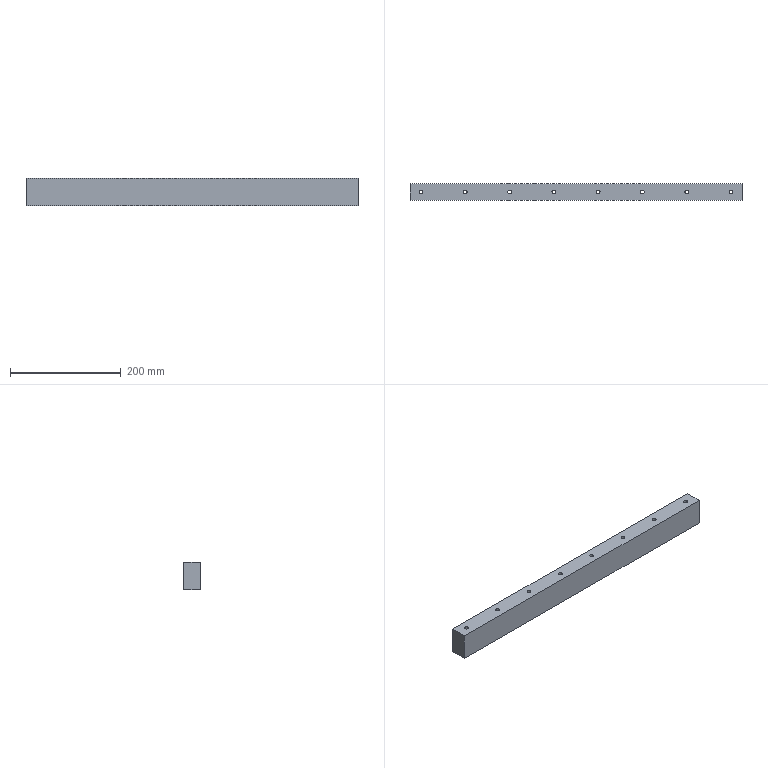Part | SolidWorks | features 3DProfileFeature 1, BaseBody 1, HoleWzd 1, LPattern 1 | 1 solid | 22 faces | box 600 x 30 x 50 mm | volume 885473 mm3 | cylinder 16 | plane 6 | commonest cylinder face diameters 6.8 x16
STEP:
#1=CARTESIAN_POINT('',(-276.6,0.,-25.));
#2=VERTEX_POINT('',#1);
#3=CARTESIAN_POINT('',(-283.4,0.,-25.));
#4=VERTEX_POINT('',#3);
#5=CARTESIAN_POINT('',(-280.,0.,-25.));
#6=DIRECTION('',(0.,0.,-1.));
#7=DIRECTION('',(1.,0.,0.));
#8=AXIS2_PLACEMENT_3D('',#5,#6,#7);
#9=CIRCLE('',#8,3.4);
#10=EDGE_CURVE('',#2,#4,#9,.T.);
#11=ORIENTED_EDGE('',*,*,#10,.T.);
#12=CARTESIAN_POINT('',(-283.4,0.,25.));
#13=VERTEX_POINT('',#12);
#14=CARTESIAN_POINT('',(-283.4,0.,-25.));
#15=DIRECTION('',(0.,0.,1.));
#16=VECTOR('',#15,1000.);
#17=LINE('',#14,#16);
#18=EDGE_CURVE('',#4,#13,#17,.T.);
#19=ORIENTED_EDGE('',*,*,#18,.T.);
#20=CARTESIAN_POINT('',(-276.6,0.,25.));
#21=VERTEX_POINT('',#20);
#22=CARTESIAN_POINT('',(-280.,0.,25.));
#23=DIRECTION('',(0.,0.,1.));
#24=DIRECTION('',(1.,0.,0.));
#25=AXIS2_PLACEMENT_3D('',#22,#23,#24);
#26=CIRCLE('',#25,3.4);
#27=EDGE_CURVE('',#13,#21,#26,.T.);
#28=ORIENTED_EDGE('',*,*,#27,.T.);
#29=CARTESIAN_POINT('',(-276.6,0.,-25.));
#30=DIRECTION('',(0.,0.,1.));
#31=VECTOR('',#30,1000.);
#32=LINE('',#29,#31);
#33=EDGE_CURVE('',#2,#21,#32,.T.);
#34=ORIENTED_EDGE('',*,*,#33,.F.);
#35=EDGE_LOOP('',(#11,#19,#28,#34));
#36=FACE_OUTER_BOUND('',#35,.T.);
#37=CARTESIAN_POINT('',(-280.,0.,-25.));
#38=DIRECTION('',(0.,0.,1.));
#39=DIRECTION('',(1.,0.,0.));
#40=AXIS2_PLACEMENT_3D('',#37,#38,#39);
#41=CYLINDRICAL_SURFACE('',#40,3.4);
#42=ADVANCED_FACE('',(#36),#41,.F.);
#43=CARTESIAN_POINT('',(276.6,0.,-25.));
#44=VERTEX_POINT('',#43);
#45=CARTESIAN_POINT('',(283.4,0.,-25.));
#46=VERTEX_POINT('',#45);
#47=CARTESIAN_POINT('',(280.,0.,-25.));
#48=DIRECTION('',(0.,0.,1.));
#49=DIRECTION('',(1.,0.,0.));
#50=AXIS2_PLACEMENT_3D('',#47,#48,#49);
#51=CIRCLE('',#50,3.4);
#52=EDGE_CURVE('',#44,#46,#51,.T.);
#53=ORIENTED_EDGE('',*,*,#52,.F.);
#54=CARTESIAN_POINT('',(276.6,0.,25.));
#55=VERTEX_POINT('',#54);
#56=CARTESIAN_POINT('',(276.6,0.,-25.));
#57=DIRECTION('',(0.,0.,1.));
#58=VECTOR('',#57,1000.);
#59=LINE('',#56,#58);
#60=EDGE_CURVE('',#44,#55,#59,.T.);
#61=ORIENTED_EDGE('',*,*,#60,.T.);
#62=CARTESIAN_POINT('',(283.4,0.,25.));
#63=VERTEX_POINT('',#62);
#64=CARTESIAN_POINT('',(280.,0.,25.));
#65=DIRECTION('',(0.,0.,1.));
#66=DIRECTION('',(1.,0.,0.));
#67=AXIS2_PLACEMENT_3D('',#64,#65,#66);
#68=CIRCLE('',#67,3.4);
#69=EDGE_CURVE('',#55,#63,#68,.T.);
#70=ORIENTED_EDGE('',*,*,#69,.T.);
#71=CARTESIAN_POINT('',(283.4,0.,-25.));
#72=DIRECTION('',(0.,0.,1.));
#73=VECTOR('',#72,1000.);
#74=LINE('',#71,#73);
#75=EDGE_CURVE('',#46,#63,#74,.T.);
#76=ORIENTED_EDGE('',*,*,#75,.F.);
#77=EDGE_LOOP('',(#53,#61,#70,#76));
#78=FACE_OUTER_BOUND('',#77,.T.);
#79=CARTESIAN_POINT('',(280.,0.,-25.));
#80=DIRECTION('',(0.,0.,1.));
#81=DIRECTION('',(1.,0.,0.));
#82=AXIS2_PLACEMENT_3D('',#79,#80,#81);
#83=CYLINDRICAL_SURFACE('',#82,3.4);
#84=ADVANCED_FACE('',(#78),#83,.F.);
#85=CARTESIAN_POINT('',(196.6,0.,-25.));
#86=VERTEX_POINT('',#85);
#87=CARTESIAN_POINT('',(203.4,0.,-25.));
#88=VERTEX_POINT('',#87);
#89=CARTESIAN_POINT('',(200.,0.,-25.));
#90=DIRECTION('',(0.,0.,1.));
#91=DIRECTION('',(1.,0.,0.));
#92=AXIS2_PLACEMENT_3D('',#89,#90,#91);
#93=CIRCLE('',#92,3.4);
#94=EDGE_CURVE('',#86,#88,#93,.T.);
#95=ORIENTED_EDGE('',*,*,#94,.F.);
#96=CARTESIAN_POINT('',(196.6,0.,25.));
#97=VERTEX_POINT('',#96);
#98=CARTESIAN_POINT('',(196.6,0.,-25.));
#99=DIRECTION('',(0.,0.,1.));
#100=VECTOR('',#99,1000.);
#101=LINE('',#98,#100);
#102=EDGE_CURVE('',#86,#97,#101,.T.);
#103=ORIENTED_EDGE('',*,*,#102,.T.);
#104=CARTESIAN_POINT('',(203.4,0.,25.));
#105=VERTEX_POINT('',#104);
#106=CARTESIAN_POINT('',(200.,0.,25.));
#107=DIRECTION('',(0.,0.,1.));
#108=DIRECTION('',(1.,0.,0.));
#109=AXIS2_PLACEMENT_3D('',#106,#107,#108);
#110=CIRCLE('',#109,3.4);
#111=EDGE_CURVE('',#97,#105,#110,.T.);
#112=ORIENTED_EDGE('',*,*,#111,.T.);
#113=CARTESIAN_POINT('',(203.4,0.,-25.));
#114=DIRECTION('',(0.,0.,1.));
#115=VECTOR('',#114,1000.);
#116=LINE('',#113,#115);
#117=EDGE_CURVE('',#88,#105,#116,.T.);
#118=ORIENTED_EDGE('',*,*,#117,.F.);
#119=EDGE_LOOP('',(#95,#103,#112,#118));
#120=FACE_OUTER_BOUND('',#119,.T.);
#121=CARTESIAN_POINT('',(200.,0.,-25.));
#122=DIRECTION('',(0.,0.,1.));
#123=DIRECTION('',(1.,0.,0.));
#124=AXIS2_PLACEMENT_3D('',#121,#122,#123);
#125=CYLINDRICAL_SURFACE('',#124,3.4);
#126=ADVANCED_FACE('',(#120),#125,.F.);
#127=CARTESIAN_POINT('',(116.6,0.,-25.));
#128=VERTEX_POINT('',#127);
#129=CARTESIAN_POINT('',(123.4,0.,-25.));
#130=VERTEX_POINT('',#129);
#131=CARTESIAN_POINT('',(120.,0.,-25.));
#132=DIRECTION('',(0.,0.,1.));
#133=DIRECTION('',(1.,0.,0.));
#134=AXIS2_PLACEMENT_3D('',#131,#132,#133);
#135=CIRCLE('',#134,3.4);
#136=EDGE_CURVE('',#128,#130,#135,.T.);
#137=ORIENTED_EDGE('',*,*,#136,.F.);
#138=CARTESIAN_POINT('',(116.6,0.,25.));
#139=VERTEX_POINT('',#138);
#140=CARTESIAN_POINT('',(116.6,0.,-25.));
#141=DIRECTION('',(0.,0.,1.));
#142=VECTOR('',#141,1000.);
#143=LINE('',#140,#142);
#144=EDGE_CURVE('',#128,#139,#143,.T.);
#145=ORIENTED_EDGE('',*,*,#144,.T.);
#146=CARTESIAN_POINT('',(123.4,0.,25.));
#147=VERTEX_POINT('',#146);
#148=CARTESIAN_POINT('',(120.,0.,25.));
#149=DIRECTION('',(0.,0.,1.));
#150=DIRECTION('',(1.,0.,0.));
#151=AXIS2_PLACEMENT_3D('',#148,#149,#150);
#152=CIRCLE('',#151,3.4);
#153=EDGE_CURVE('',#139,#147,#152,.T.);
#154=ORIENTED_EDGE('',*,*,#153,.T.);
#155=CARTESIAN_POINT('',(123.4,0.,-25.));
#156=DIRECTION('',(0.,0.,1.));
#157=VECTOR('',#156,1000.);
#158=LINE('',#155,#157);
#159=EDGE_CURVE('',#130,#147,#158,.T.);
#160=ORIENTED_EDGE('',*,*,#159,.F.);
#161=EDGE_LOOP('',(#137,#145,#154,#160));
#162=FACE_OUTER_BOUND('',#161,.T.);
#163=CARTESIAN_POINT('',(120.,0.,-25.));
#164=DIRECTION('',(0.,0.,1.));
#165=DIRECTION('',(1.,0.,0.));
#166=AXIS2_PLACEMENT_3D('',#163,#164,#165);
#167=CYLINDRICAL_SURFACE('',#166,3.4);
#168=ADVANCED_FACE('',(#162),#167,.F.);
#169=CARTESIAN_POINT('',(36.6,0.,-25.));
#170=VERTEX_POINT('',#169);
#171=CARTESIAN_POINT('',(43.4,0.,-25.));
#172=VERTEX_POINT('',#171);
#173=CARTESIAN_POINT('',(40.,0.,-25.));
#174=DIRECTION('',(0.,0.,1.));
#175=DIRECTION('',(1.,0.,0.));
#176=AXIS2_PLACEMENT_3D('',#173,#174,#175);
#177=CIRCLE('',#176,3.4);
#178=EDGE_CURVE('',#170,#172,#177,.T.);
#179=ORIENTED_EDGE('',*,*,#178,.F.);
#180=CARTESIAN_POINT('',(36.6,0.,25.));
#181=VERTEX_POINT('',#180);
#182=CARTESIAN_POINT('',(36.6,0.,-25.));
#183=DIRECTION('',(0.,0.,1.));
#184=VECTOR('',#183,1000.);
#185=LINE('',#182,#184);
#186=EDGE_CURVE('',#170,#181,#185,.T.);
#187=ORIENTED_EDGE('',*,*,#186,.T.);
#188=CARTESIAN_POINT('',(43.4,0.,25.));
#189=VERTEX_POINT('',#188);
#190=CARTESIAN_POINT('',(40.,0.,25.));
#191=DIRECTION('',(0.,0.,1.));
#192=DIRECTION('',(1.,0.,0.));
#193=AXIS2_PLACEMENT_3D('',#190,#191,#192);
#194=CIRCLE('',#193,3.4);
#195=EDGE_CURVE('',#181,#189,#194,.T.);
#196=ORIENTED_EDGE('',*,*,#195,.T.);
#197=CARTESIAN_POINT('',(43.4,0.,-25.));
#198=DIRECTION('',(0.,0.,1.));
#199=VECTOR('',#198,1000.);
#200=LINE('',#197,#199);
#201=EDGE_CURVE('',#172,#189,#200,.T.);
#202=ORIENTED_EDGE('',*,*,#201,.F.);
#203=EDGE_LOOP('',(#179,#187,#196,#202));
#204=FACE_OUTER_BOUND('',#203,.T.);
#205=CARTESIAN_POINT('',(40.,0.,-25.));
#206=DIRECTION('',(0.,0.,1.));
#207=DIRECTION('',(1.,0.,0.));
#208=AXIS2_PLACEMENT_3D('',#205,#206,#207);
#209=CYLINDRICAL_SURFACE('',#208,3.4);
#210=ADVANCED_FACE('',(#204),#209,.F.);
#211=CARTESIAN_POINT('',(-43.4,0.,-25.));
#212=VERTEX_POINT('',#211);
#213=CARTESIAN_POINT('',(-36.6,0.,-25.));
#214=VERTEX_POINT('',#213);
#215=CARTESIAN_POINT('',(-40.,0.,-25.));
#216=DIRECTION('',(0.,0.,1.));
#217=DIRECTION('',(1.,0.,0.));
#218=AXIS2_PLACEMENT_3D('',#215,#216,#217);
#219=CIRCLE('',#218,3.4);
#220=EDGE_CURVE('',#212,#214,#219,.T.);
#221=ORIENTED_EDGE('',*,*,#220,.F.);
#222=CARTESIAN_POINT('',(-43.4,0.,25.));
#223=VERTEX_POINT('',#222);
#224=CARTESIAN_POINT('',(-43.4,0.,-25.));
#225=DIRECTION('',(0.,0.,1.));
#226=VECTOR('',#225,1000.);
#227=LINE('',#224,#226);
#228=EDGE_CURVE('',#212,#223,#227,.T.);
#229=ORIENTED_EDGE('',*,*,#228,.T.);
#230=CARTESIAN_POINT('',(-36.6,0.,25.));
#231=VERTEX_POINT('',#230);
#232=CARTESIAN_POINT('',(-40.,0.,25.));
#233=DIRECTION('',(0.,0.,1.));
#234=DIRECTION('',(1.,0.,0.));
#235=AXIS2_PLACEMENT_3D('',#232,#233,#234);
#236=CIRCLE('',#235,3.4);
#237=EDGE_CURVE('',#223,#231,#236,.T.);
#238=ORIENTED_EDGE('',*,*,#237,.T.);
#239=CARTESIAN_POINT('',(-36.6,0.,-25.));
#240=DIRECTION('',(0.,0.,1.));
#241=VECTOR('',#240,1000.);
#242=LINE('',#239,#241);
#243=EDGE_CURVE('',#214,#231,#242,.T.);
#244=ORIENTED_EDGE('',*,*,#243,.F.);
#245=EDGE_LOOP('',(#221,#229,#238,#244));
#246=FACE_OUTER_BOUND('',#245,.T.);
#247=CARTESIAN_POINT('',(-40.,0.,-25.));
#248=DIRECTION('',(0.,0.,1.));
#249=DIRECTION('',(1.,0.,0.));
#250=AXIS2_PLACEMENT_3D('',#247,#248,#249);
#251=CYLINDRICAL_SURFACE('',#250,3.4);
#252=ADVANCED_FACE('',(#246),#251,.F.);
#253=CARTESIAN_POINT('',(-123.4,0.,-25.));
#254=VERTEX_POINT('',#253);
#255=CARTESIAN_POINT('',(-116.6,0.,-25.));
#256=VERTEX_POINT('',#255);
#257=CARTESIAN_POINT('',(-120.,0.,-25.));
#258=DIRECTION('',(0.,0.,1.));
#259=DIRECTION('',(1.,0.,0.));
#260=AXIS2_PLACEMENT_3D('',#257,#258,#259);
#261=CIRCLE('',#260,3.4);
#262=EDGE_CURVE('',#254,#256,#261,.T.);
#263=ORIENTED_EDGE('',*,*,#262,.F.);
#264=CARTESIAN_POINT('',(-123.4,0.,25.));
#265=VERTEX_POINT('',#264);
#266=CARTESIAN_POINT('',(-123.4,0.,-25.));
#267=DIRECTION('',(0.,0.,1.));
#268=VECTOR('',#267,1000.);
#269=LINE('',#266,#268);
#270=EDGE_CURVE('',#254,#265,#269,.T.);
#271=ORIENTED_EDGE('',*,*,#270,.T.);
#272=CARTESIAN_POINT('',(-116.6,0.,25.));
#273=VERTEX_POINT('',#272);
#274=CARTESIAN_POINT('',(-120.,0.,25.));
#275=DIRECTION('',(0.,0.,1.));
#276=DIRECTION('',(1.,0.,0.));
#277=AXIS2_PLACEMENT_3D('',#274,#275,#276);
#278=CIRCLE('',#277,3.4);
#279=EDGE_CURVE('',#265,#273,#278,.T.);
#280=ORIENTED_EDGE('',*,*,#279,.T.);
#281=CARTESIAN_POINT('',(-116.6,0.,-25.));
#282=DIRECTION('',(0.,0.,1.));
#283=VECTOR('',#282,1000.);
#284=LINE('',#281,#283);
#285=EDGE_CURVE('',#256,#273,#284,.T.);
#286=ORIENTED_EDGE('',*,*,#285,.F.);
#287=EDGE_LOOP('',(#263,#271,#280,#286));
#288=FACE_OUTER_BOUND('',#287,.T.);
#289=CARTESIAN_POINT('',(-120.,0.,-25.));
#290=DIRECTION('',(0.,0.,1.));
#291=DIRECTION('',(1.,0.,0.));
#292=AXIS2_PLACEMENT_3D('',#289,#290,#291);
#293=CYLINDRICAL_SURFACE('',#292,3.4);
#294=ADVANCED_FACE('',(#288),#293,.F.);
#295=CARTESIAN_POINT('',(-203.4,0.,-25.));
#296=VERTEX_POINT('',#295);
#297=CARTESIAN_POINT('',(-196.6,0.,-25.));
#298=VERTEX_POINT('',#297);
#299=CARTESIAN_POINT('',(-200.,0.,-25.));
#300=DIRECTION('',(0.,0.,1.));
#301=DIRECTION('',(1.,0.,0.));
#302=AXIS2_PLACEMENT_3D('',#299,#300,#301);
#303=CIRCLE('',#302,3.4);
#304=EDGE_CURVE('',#296,#298,#303,.T.);
#305=ORIENTED_EDGE('',*,*,#304,.F.);
#306=CARTESIAN_POINT('',(-203.4,0.,25.));
#307=VERTEX_POINT('',#306);
#308=CARTESIAN_POINT('',(-203.4,0.,-25.));
#309=DIRECTION('',(0.,0.,1.));
#310=VECTOR('',#309,1000.);
#311=LINE('',#308,#310);
#312=EDGE_CURVE('',#296,#307,#311,.T.);
#313=ORIENTED_EDGE('',*,*,#312,.T.);
#314=CARTESIAN_POINT('',(-196.6,0.,25.));
#315=VERTEX_POINT('',#314);
#316=CARTESIAN_POINT('',(-200.,0.,25.));
#317=DIRECTION('',(0.,0.,1.));
#318=DIRECTION('',(1.,0.,0.));
#319=AXIS2_PLACEMENT_3D('',#316,#317,#318);
#320=CIRCLE('',#319,3.4);
#321=EDGE_CURVE('',#307,#315,#320,.T.);
#322=ORIENTED_EDGE('',*,*,#321,.T.);
#323=CARTESIAN_POINT('',(-196.6,0.,-25.));
#324=DIRECTION('',(0.,0.,1.));
#325=VECTOR('',#324,1000.);
#326=LINE('',#323,#325);
#327=EDGE_CURVE('',#298,#315,#326,.T.);
#328=ORIENTED_EDGE('',*,*,#327,.F.);
#329=EDGE_LOOP('',(#305,#313,#322,#328));
#330=FACE_OUTER_BOUND('',#329,.T.);
#331=CARTESIAN_POINT('',(-200.,0.,-25.));
#332=DIRECTION('',(0.,0.,1.));
#333=DIRECTION('',(1.,0.,0.));
#334=AXIS2_PLACEMENT_3D('',#331,#332,#333);
#335=CYLINDRICAL_SURFACE('',#334,3.4);
#336=ADVANCED_FACE('',(#330),#335,.F.);
#337=ORIENTED_EDGE('',*,*,#18,.F.);
#338=CARTESIAN_POINT('',(-280.,0.,-25.));
#339=DIRECTION('',(0.,0.,-1.));
#340=DIRECTION('',(1.,0.,0.));
#341=AXIS2_PLACEMENT_3D('',#338,#339,#340);
#342=CIRCLE('',#341,3.4);
#343=EDGE_CURVE('',#4,#2,#342,.T.);
#344=ORIENTED_EDGE('',*,*,#343,.T.);
#345=ORIENTED_EDGE('',*,*,#33,.T.);
#346=CARTESIAN_POINT('',(-280.,0.,25.));
#347=DIRECTION('',(0.,0.,1.));
#348=DIRECTION('',(1.,0.,0.));
#349=AXIS2_PLACEMENT_3D('',#346,#347,#348);
#350=CIRCLE('',#349,3.4);
#351=EDGE_CURVE('',#21,#13,#350,.T.);
#352=ORIENTED_EDGE('',*,*,#351,.T.);
#353=EDGE_LOOP('',(#337,#344,#345,#352));
#354=FACE_OUTER_BOUND('',#353,.T.);
#355=CARTESIAN_POINT('',(-280.,0.,-25.));
#356=DIRECTION('',(0.,0.,1.));
#357=DIRECTION('',(1.,0.,0.));
#358=AXIS2_PLACEMENT_3D('',#355,#356,#357);
#359=CYLINDRICAL_SURFACE('',#358,3.4);
#360=ADVANCED_FACE('',(#354),#359,.F.);
#361=CARTESIAN_POINT('',(280.,0.,25.));
#362=DIRECTION('',(0.,0.,1.));
#363=DIRECTION('',(1.,0.,0.));
#364=AXIS2_PLACEMENT_3D('',#361,#362,#363);
#365=CIRCLE('',#364,3.4);
#366=EDGE_CURVE('',#63,#55,#365,.T.);
#367=ORIENTED_EDGE('',*,*,#366,.F.);
#368=ORIENTED_EDGE('',*,*,#69,.F.);
#369=EDGE_LOOP('',(#367,#368));
#370=FACE_BOUND('',#369,.T.);
#371=CARTESIAN_POINT('',(200.,0.,25.));
#372=DIRECTION('',(0.,0.,1.));
#373=DIRECTION('',(1.,0.,0.));
#374=AXIS2_PLACEMENT_3D('',#371,#372,#373);
#375=CIRCLE('',#374,3.4);
#376=EDGE_CURVE('',#105,#97,#375,.T.);
#377=ORIENTED_EDGE('',*,*,#376,.F.);
#378=ORIENTED_EDGE('',*,*,#111,.F.);
#379=EDGE_LOOP('',(#377,#378));
#380=FACE_BOUND('',#379,.T.);
#381=CARTESIAN_POINT('',(120.,0.,25.));
#382=DIRECTION('',(0.,0.,1.));
#383=DIRECTION('',(1.,0.,0.));
#384=AXIS2_PLACEMENT_3D('',#381,#382,#383);
#385=CIRCLE('',#384,3.4);
#386=EDGE_CURVE('',#147,#139,#385,.T.);
#387=ORIENTED_EDGE('',*,*,#386,.F.);
#388=ORIENTED_EDGE('',*,*,#153,.F.);
#389=EDGE_LOOP('',(#387,#388));
#390=FACE_BOUND('',#389,.T.);
#391=CARTESIAN_POINT('',(40.,0.,25.));
#392=DIRECTION('',(0.,0.,1.));
#393=DIRECTION('',(1.,0.,0.));
#394=AXIS2_PLACEMENT_3D('',#391,#392,#393);
#395=CIRCLE('',#394,3.4);
#396=EDGE_CURVE('',#189,#181,#395,.T.);
#397=ORIENTED_EDGE('',*,*,#396,.F.);
#398=ORIENTED_EDGE('',*,*,#195,.F.);
#399=EDGE_LOOP('',(#397,#398));
#400=FACE_BOUND('',#399,.T.);
#401=CARTESIAN_POINT('',(-40.,0.,25.));
#402=DIRECTION('',(0.,0.,1.));
#403=DIRECTION('',(1.,0.,0.));
#404=AXIS2_PLACEMENT_3D('',#401,#402,#403);
#405=CIRCLE('',#404,3.4);
#406=EDGE_CURVE('',#231,#223,#405,.T.);
#407=ORIENTED_EDGE('',*,*,#406,.F.);
#408=ORIENTED_EDGE('',*,*,#237,.F.);
#409=EDGE_LOOP('',(#407,#408));
#410=FACE_BOUND('',#409,.T.);
#411=CARTESIAN_POINT('',(-120.,0.,25.));
#412=DIRECTION('',(0.,0.,1.));
#413=DIRECTION('',(1.,0.,0.));
#414=AXIS2_PLACEMENT_3D('',#411,#412,#413);
#415=CIRCLE('',#414,3.4);
#416=EDGE_CURVE('',#273,#265,#415,.T.);
#417=ORIENTED_EDGE('',*,*,#416,.F.);
#418=ORIENTED_EDGE('',*,*,#279,.F.);
#419=EDGE_LOOP('',(#417,#418));
#420=FACE_BOUND('',#419,.T.);
#421=CARTESIAN_POINT('',(-200.,0.,25.));
#422=DIRECTION('',(0.,0.,1.));
#423=DIRECTION('',(1.,0.,0.));
#424=AXIS2_PLACEMENT_3D('',#421,#422,#423);
#425=CIRCLE('',#424,3.4);
#426=EDGE_CURVE('',#315,#307,#425,.T.);
#427=ORIENTED_EDGE('',*,*,#426,.F.);
#428=ORIENTED_EDGE('',*,*,#321,.F.);
#429=EDGE_LOOP('',(#427,#428));
#430=FACE_BOUND('',#429,.T.);
#431=ORIENTED_EDGE('',*,*,#351,.F.);
#432=ORIENTED_EDGE('',*,*,#27,.F.);
#433=EDGE_LOOP('',(#431,#432));
#434=FACE_BOUND('',#433,.T.);
#435=CARTESIAN_POINT('',(-300.,15.,25.));
#436=VERTEX_POINT('',#435);
#437=CARTESIAN_POINT('',(300.,15.,25.));
#438=VERTEX_POINT('',#437);
#439=CARTESIAN_POINT('',(0.,15.,25.));
#440=DIRECTION('',(1.,0.,0.));
#441=VECTOR('',#440,1000.);
#442=LINE('',#439,#441);
#443=EDGE_CURVE('',#436,#438,#442,.T.);
#444=ORIENTED_EDGE('',*,*,#443,.F.);
#445=CARTESIAN_POINT('',(-300.,-15.,25.));
#446=VERTEX_POINT('',#445);
#447=CARTESIAN_POINT('',(-300.,0.,25.));
#448=DIRECTION('',(0.,1.,0.));
#449=VECTOR('',#448,1000.);
#450=LINE('',#447,#449);
#451=EDGE_CURVE('',#446,#436,#450,.T.);
#452=ORIENTED_EDGE('',*,*,#451,.F.);
#453=CARTESIAN_POINT('',(300.,-15.,25.));
#454=VERTEX_POINT('',#453);
#455=CARTESIAN_POINT('',(0.,-15.,25.));
#456=DIRECTION('',(-1.,0.,0.));
#457=VECTOR('',#456,1000.);
#458=LINE('',#455,#457);
#459=EDGE_CURVE('',#454,#446,#458,.T.);
#460=ORIENTED_EDGE('',*,*,#459,.F.);
#461=CARTESIAN_POINT('',(300.,0.,25.));
#462=DIRECTION('',(0.,-1.,0.));
#463=VECTOR('',#462,1000.);
#464=LINE('',#461,#463);
#465=EDGE_CURVE('',#438,#454,#464,.T.);
#466=ORIENTED_EDGE('',*,*,#465,.F.);
#467=EDGE_LOOP('',(#444,#452,#460,#466));
#468=FACE_OUTER_BOUND('',#467,.T.);
#469=CARTESIAN_POINT('',(300.,-15.,25.));
#470=DIRECTION('',(0.,0.,-1.));
#471=DIRECTION('',(-1.,0.,0.));
#472=AXIS2_PLACEMENT_3D('',#469,#470,#471);
#473=PLANE('',#472);
#474=ADVANCED_FACE('',(#370,#380,#390,#400,#410,#420,#430,#434,#468),#473,.F.);
#475=CARTESIAN_POINT('',(280.,0.,-25.));
#476=DIRECTION('',(0.,0.,1.));
#477=DIRECTION('',(1.,0.,0.));
#478=AXIS2_PLACEMENT_3D('',#475,#476,#477);
#479=CIRCLE('',#478,3.4);
#480=EDGE_CURVE('',#46,#44,#479,.T.);
#481=ORIENTED_EDGE('',*,*,#480,.T.);
#482=ORIENTED_EDGE('',*,*,#52,.T.);
#483=EDGE_LOOP('',(#481,#482));
#484=FACE_BOUND('',#483,.T.);
#485=CARTESIAN_POINT('',(200.,0.,-25.));
#486=DIRECTION('',(0.,0.,1.));
#487=DIRECTION('',(1.,0.,0.));
#488=AXIS2_PLACEMENT_3D('',#485,#486,#487);
#489=CIRCLE('',#488,3.4);
#490=EDGE_CURVE('',#88,#86,#489,.T.);
#491=ORIENTED_EDGE('',*,*,#490,.T.);
#492=ORIENTED_EDGE('',*,*,#94,.T.);
#493=EDGE_LOOP('',(#491,#492));
#494=FACE_BOUND('',#493,.T.);
#495=CARTESIAN_POINT('',(120.,0.,-25.));
#496=DIRECTION('',(0.,0.,1.));
#497=DIRECTION('',(1.,0.,0.));
#498=AXIS2_PLACEMENT_3D('',#495,#496,#497);
#499=CIRCLE('',#498,3.4);
#500=EDGE_CURVE('',#130,#128,#499,.T.);
#501=ORIENTED_EDGE('',*,*,#500,.T.);
#502=ORIENTED_EDGE('',*,*,#136,.T.);
#503=EDGE_LOOP('',(#501,#502));
#504=FACE_BOUND('',#503,.T.);
#505=CARTESIAN_POINT('',(40.,0.,-25.));
#506=DIRECTION('',(0.,0.,1.));
#507=DIRECTION('',(1.,0.,0.));
#508=AXIS2_PLACEMENT_3D('',#505,#506,#507);
#509=CIRCLE('',#508,3.4);
#510=EDGE_CURVE('',#172,#170,#509,.T.);
#511=ORIENTED_EDGE('',*,*,#510,.T.);
#512=ORIENTED_EDGE('',*,*,#178,.T.);
#513=EDGE_LOOP('',(#511,#512));
#514=FACE_BOUND('',#513,.T.);
#515=CARTESIAN_POINT('',(-40.,0.,-25.));
#516=DIRECTION('',(0.,0.,1.));
#517=DIRECTION('',(1.,0.,0.));
#518=AXIS2_PLACEMENT_3D('',#515,#516,#517);
#519=CIRCLE('',#518,3.4);
#520=EDGE_CURVE('',#214,#212,#519,.T.);
#521=ORIENTED_EDGE('',*,*,#520,.T.);
#522=ORIENTED_EDGE('',*,*,#220,.T.);
#523=EDGE_LOOP('',(#521,#522));
#524=FACE_BOUND('',#523,.T.);
#525=CARTESIAN_POINT('',(-120.,0.,-25.));
#526=DIRECTION('',(0.,0.,1.));
#527=DIRECTION('',(1.,0.,0.));
#528=AXIS2_PLACEMENT_3D('',#525,#526,#527);
#529=CIRCLE('',#528,3.4);
#530=EDGE_CURVE('',#256,#254,#529,.T.);
#531=ORIENTED_EDGE('',*,*,#530,.T.);
#532=ORIENTED_EDGE('',*,*,#262,.T.);
#533=EDGE_LOOP('',(#531,#532));
#534=FACE_BOUND('',#533,.T.);
#535=CARTESIAN_POINT('',(-200.,0.,-25.));
#536=DIRECTION('',(0.,0.,1.));
#537=DIRECTION('',(1.,0.,0.));
#538=AXIS2_PLACEMENT_3D('',#535,#536,#537);
#539=CIRCLE('',#538,3.4);
#540=EDGE_CURVE('',#298,#296,#539,.T.);
#541=ORIENTED_EDGE('',*,*,#540,.T.);
#542=ORIENTED_EDGE('',*,*,#304,.T.);
#543=EDGE_LOOP('',(#541,#542));
#544=FACE_BOUND('',#543,.T.);
#545=ORIENTED_EDGE('',*,*,#10,.F.);
#546=ORIENTED_EDGE('',*,*,#343,.F.);
#547=EDGE_LOOP('',(#545,#546));
#548=FACE_BOUND('',#547,.T.);
#549=CARTESIAN_POINT('',(-300.,-15.,-25.));
#550=VERTEX_POINT('',#549);
#551=CARTESIAN_POINT('',(-300.,15.,-25.));
#552=VERTEX_POINT('',#551);
#553=CARTESIAN_POINT('',(-300.,0.,-25.));
#554=DIRECTION('',(0.,1.,0.));
#555=VECTOR('',#554,1000.);
#556=LINE('',#553,#555);
#557=EDGE_CURVE('',#550,#552,#556,.T.);
#558=ORIENTED_EDGE('',*,*,#557,.T.);
#559=CARTESIAN_POINT('',(300.,15.,-25.));
#560=VERTEX_POINT('',#559);
#561=CARTESIAN_POINT('',(0.,15.,-25.));
#562=DIRECTION('',(1.,0.,0.));
#563=VECTOR('',#562,1000.);
#564=LINE('',#561,#563);
#565=EDGE_CURVE('',#552,#560,#564,.T.);
#566=ORIENTED_EDGE('',*,*,#565,.T.);
#567=CARTESIAN_POINT('',(300.,-15.,-25.));
#568=VERTEX_POINT('',#567);
#569=CARTESIAN_POINT('',(300.,0.,-25.));
#570=DIRECTION('',(0.,-1.,0.));
#571=VECTOR('',#570,1000.);
#572=LINE('',#569,#571);
#573=EDGE_CURVE('',#560,#568,#572,.T.);
#574=ORIENTED_EDGE('',*,*,#573,.T.);
#575=CARTESIAN_POINT('',(0.,-15.,-25.));
#576=DIRECTION('',(-1.,0.,0.));
#577=VECTOR('',#576,1000.);
#578=LINE('',#575,#577);
#579=EDGE_CURVE('',#568,#550,#578,.T.);
#580=ORIENTED_EDGE('',*,*,#579,.T.);
#581=EDGE_LOOP('',(#558,#566,#574,#580));
#582=FACE_OUTER_BOUND('',#581,.T.);
#583=CARTESIAN_POINT('',(300.,-15.,-25.));
#584=DIRECTION('',(0.,0.,-1.));
#585=DIRECTION('',(-1.,0.,0.));
#586=AXIS2_PLACEMENT_3D('',#583,#584,#585);
#587=PLANE('',#586);
#588=ADVANCED_FACE('',(#484,#494,#504,#514,#524,#534,#544,#548,#582),#587,.T.);
#589=ORIENTED_EDGE('',*,*,#60,.F.);
#590=ORIENTED_EDGE('',*,*,#480,.F.);
#591=ORIENTED_EDGE('',*,*,#75,.T.);
#592=ORIENTED_EDGE('',*,*,#366,.T.);
#593=EDGE_LOOP('',(#589,#590,#591,#592));
#594=FACE_OUTER_BOUND('',#593,.T.);
#595=CARTESIAN_POINT('',(280.,0.,-25.));
#596=DIRECTION('',(0.,0.,1.));
#597=DIRECTION('',(1.,0.,0.));
#598=AXIS2_PLACEMENT_3D('',#595,#596,#597);
#599=CYLINDRICAL_SURFACE('',#598,3.4);
#600=ADVANCED_FACE('',(#594),#599,.F.);
#601=ORIENTED_EDGE('',*,*,#102,.F.);
#602=ORIENTED_EDGE('',*,*,#490,.F.);
#603=ORIENTED_EDGE('',*,*,#117,.T.);
#604=ORIENTED_EDGE('',*,*,#376,.T.);
#605=EDGE_LOOP('',(#601,#602,#603,#604));
#606=FACE_OUTER_BOUND('',#605,.T.);
#607=CARTESIAN_POINT('',(200.,0.,-25.));
#608=DIRECTION('',(0.,0.,1.));
#609=DIRECTION('',(1.,0.,0.));
#610=AXIS2_PLACEMENT_3D('',#607,#608,#609);
#611=CYLINDRICAL_SURFACE('',#610,3.4);
#612=ADVANCED_FACE('',(#606),#611,.F.);
#613=ORIENTED_EDGE('',*,*,#144,.F.);
#614=ORIENTED_EDGE('',*,*,#500,.F.);
#615=ORIENTED_EDGE('',*,*,#159,.T.);
#616=ORIENTED_EDGE('',*,*,#386,.T.);
#617=EDGE_LOOP('',(#613,#614,#615,#616));
#618=FACE_OUTER_BOUND('',#617,.T.);
#619=CARTESIAN_POINT('',(120.,0.,-25.));
#620=DIRECTION('',(0.,0.,1.));
#621=DIRECTION('',(1.,0.,0.));
#622=AXIS2_PLACEMENT_3D('',#619,#620,#621);
#623=CYLINDRICAL_SURFACE('',#622,3.4);
#624=ADVANCED_FACE('',(#618),#623,.F.);
#625=ORIENTED_EDGE('',*,*,#186,.F.);
#626=ORIENTED_EDGE('',*,*,#510,.F.);
#627=ORIENTED_EDGE('',*,*,#201,.T.);
#628=ORIENTED_EDGE('',*,*,#396,.T.);
#629=EDGE_LOOP('',(#625,#626,#627,#628));
#630=FACE_OUTER_BOUND('',#629,.T.);
#631=CARTESIAN_POINT('',(40.,0.,-25.));
#632=DIRECTION('',(0.,0.,1.));
#633=DIRECTION('',(1.,0.,0.));
#634=AXIS2_PLACEMENT_3D('',#631,#632,#633);
#635=CYLINDRICAL_SURFACE('',#634,3.4);
#636=ADVANCED_FACE('',(#630),#635,.F.);
#637=ORIENTED_EDGE('',*,*,#228,.F.);
#638=ORIENTED_EDGE('',*,*,#520,.F.);
#639=ORIENTED_EDGE('',*,*,#243,.T.);
#640=ORIENTED_EDGE('',*,*,#406,.T.);
#641=EDGE_LOOP('',(#637,#638,#639,#640));
#642=FACE_OUTER_BOUND('',#641,.T.);
#643=CARTESIAN_POINT('',(-40.,0.,-25.));
#644=DIRECTION('',(0.,0.,1.));
#645=DIRECTION('',(1.,0.,0.));
#646=AXIS2_PLACEMENT_3D('',#643,#644,#645);
#647=CYLINDRICAL_SURFACE('',#646,3.4);
#648=ADVANCED_FACE('',(#642),#647,.F.);
#649=ORIENTED_EDGE('',*,*,#270,.F.);
#650=ORIENTED_EDGE('',*,*,#530,.F.);
#651=ORIENTED_EDGE('',*,*,#285,.T.);
#652=ORIENTED_EDGE('',*,*,#416,.T.);
#653=EDGE_LOOP('',(#649,#650,#651,#652));
#654=FACE_OUTER_BOUND('',#653,.T.);
#655=CARTESIAN_POINT('',(-120.,0.,-25.));
#656=DIRECTION('',(0.,0.,1.));
#657=DIRECTION('',(1.,0.,0.));
#658=AXIS2_PLACEMENT_3D('',#655,#656,#657);
#659=CYLINDRICAL_SURFACE('',#658,3.4);
#660=ADVANCED_FACE('',(#654),#659,.F.);
#661=ORIENTED_EDGE('',*,*,#312,.F.);
#662=ORIENTED_EDGE('',*,*,#540,.F.);
#663=ORIENTED_EDGE('',*,*,#327,.T.);
#664=ORIENTED_EDGE('',*,*,#426,.T.);
#665=EDGE_LOOP('',(#661,#662,#663,#664));
#666=FACE_OUTER_BOUND('',#665,.T.);
#667=CARTESIAN_POINT('',(-200.,0.,-25.));
#668=DIRECTION('',(0.,0.,1.));
#669=DIRECTION('',(1.,0.,0.));
#670=AXIS2_PLACEMENT_3D('',#667,#668,#669);
#671=CYLINDRICAL_SURFACE('',#670,3.4);
#672=ADVANCED_FACE('',(#666),#671,.F.);
#673=CARTESIAN_POINT('',(300.,15.,0.));
#674=DIRECTION('',(0.,0.,-1.));
#675=VECTOR('',#674,1000.);
#676=LINE('',#673,#675);
#677=EDGE_CURVE('',#438,#560,#676,.T.);
#678=ORIENTED_EDGE('',*,*,#677,.F.);
#679=ORIENTED_EDGE('',*,*,#465,.T.);
#680=CARTESIAN_POINT('',(300.,-15.,0.));
#681=DIRECTION('',(0.,0.,1.));
#682=VECTOR('',#681,1000.);
#683=LINE('',#680,#682);
#684=EDGE_CURVE('',#568,#454,#683,.T.);
#685=ORIENTED_EDGE('',*,*,#684,.F.);
#686=ORIENTED_EDGE('',*,*,#573,.F.);
#687=EDGE_LOOP('',(#678,#679,#685,#686));
#688=FACE_OUTER_BOUND('',#687,.T.);
#689=CARTESIAN_POINT('',(300.,-15.,-25.));
#690=DIRECTION('',(-1.,0.,0.));
#691=DIRECTION('',(0.,0.,1.));
#692=AXIS2_PLACEMENT_3D('',#689,#690,#691);
#693=PLANE('',#692);
#694=ADVANCED_FACE('',(#688),#693,.F.);
#695=CARTESIAN_POINT('',(-300.,15.,0.));
#696=DIRECTION('',(0.,0.,-1.));
#697=VECTOR('',#696,1000.);
#698=LINE('',#695,#697);
#699=EDGE_CURVE('',#436,#552,#698,.T.);
#700=ORIENTED_EDGE('',*,*,#699,.F.);
#701=ORIENTED_EDGE('',*,*,#443,.T.);
#702=ORIENTED_EDGE('',*,*,#677,.T.);
#703=ORIENTED_EDGE('',*,*,#565,.F.);
#704=EDGE_LOOP('',(#700,#701,#702,#703));
#705=FACE_OUTER_BOUND('',#704,.T.);
#706=CARTESIAN_POINT('',(-300.,15.,25.));
#707=DIRECTION('',(0.,-1.,0.));
#708=DIRECTION('',(0.,0.,-1.));
#709=AXIS2_PLACEMENT_3D('',#706,#707,#708);
#710=PLANE('',#709);
#711=ADVANCED_FACE('',(#705),#710,.F.);
#712=CARTESIAN_POINT('',(-300.,-15.,0.));
#713=DIRECTION('',(0.,0.,-1.));
#714=VECTOR('',#713,1000.);
#715=LINE('',#712,#714);
#716=EDGE_CURVE('',#446,#550,#715,.T.);
#717=ORIENTED_EDGE('',*,*,#716,.F.);
#718=ORIENTED_EDGE('',*,*,#451,.T.);
#719=ORIENTED_EDGE('',*,*,#699,.T.);
#720=ORIENTED_EDGE('',*,*,#557,.F.);
#721=EDGE_LOOP('',(#717,#718,#719,#720));
#722=FACE_OUTER_BOUND('',#721,.T.);
#723=CARTESIAN_POINT('',(-300.,-15.,25.));
#724=DIRECTION('',(1.,0.,0.));
#725=DIRECTION('',(0.,0.,-1.));
#726=AXIS2_PLACEMENT_3D('',#723,#724,#725);
#727=PLANE('',#726);
#728=ADVANCED_FACE('',(#722),#727,.F.);
#729=ORIENTED_EDGE('',*,*,#684,.T.);
#730=ORIENTED_EDGE('',*,*,#459,.T.);
#731=ORIENTED_EDGE('',*,*,#716,.T.);
#732=ORIENTED_EDGE('',*,*,#579,.F.);
#733=EDGE_LOOP('',(#729,#730,#731,#732));
#734=FACE_OUTER_BOUND('',#733,.T.);
#735=CARTESIAN_POINT('',(-300.,-15.,-25.));
#736=DIRECTION('',(0.,1.,0.));
#737=DIRECTION('',(0.,0.,1.));
#738=AXIS2_PLACEMENT_3D('',#735,#736,#737);
#739=PLANE('',#738);
#740=ADVANCED_FACE('',(#734),#739,.F.);
#741=CLOSED_SHELL('',(#42,#84,#126,#168,#210,#252,#294,#336,#360,#474,#588,#600,#612,#624,#636,#648,#660,#672,#694,#711,#728,#740));
#742=MANIFOLD_SOLID_BREP('',#741);
#743=CARTESIAN_POINT('',(0.,0.,0.));
#744=DIRECTION('',(0.,0.,1.));
#745=DIRECTION('',(1.,0.,0.));
#746=AXIS2_PLACEMENT_3D('',#743,#744,#745);
#747=(LENGTH_UNIT()NAMED_UNIT(*)SI_UNIT(.MILLI.,.METRE.));
#748=UNCERTAINTY_MEASURE_WITH_UNIT(LENGTH_MEASURE(0.00001),#747,'','');
#749=(NAMED_UNIT(*)PLANE_ANGLE_UNIT()SI_UNIT($,.RADIAN.));
#750=(NAMED_UNIT(*)SI_UNIT($,.STERADIAN.)SOLID_ANGLE_UNIT());
#751=(GEOMETRIC_REPRESENTATION_CONTEXT(3)GLOBAL_UNCERTAINTY_ASSIGNED_CONTEXT((#748))GLOBAL_UNIT_ASSIGNED_CONTEXT((#747,#749,#750))REPRESENTATION_CONTEXT('',''));
#752=ADVANCED_BREP_SHAPE_REPRESENTATION('',(#742,#746),#751);